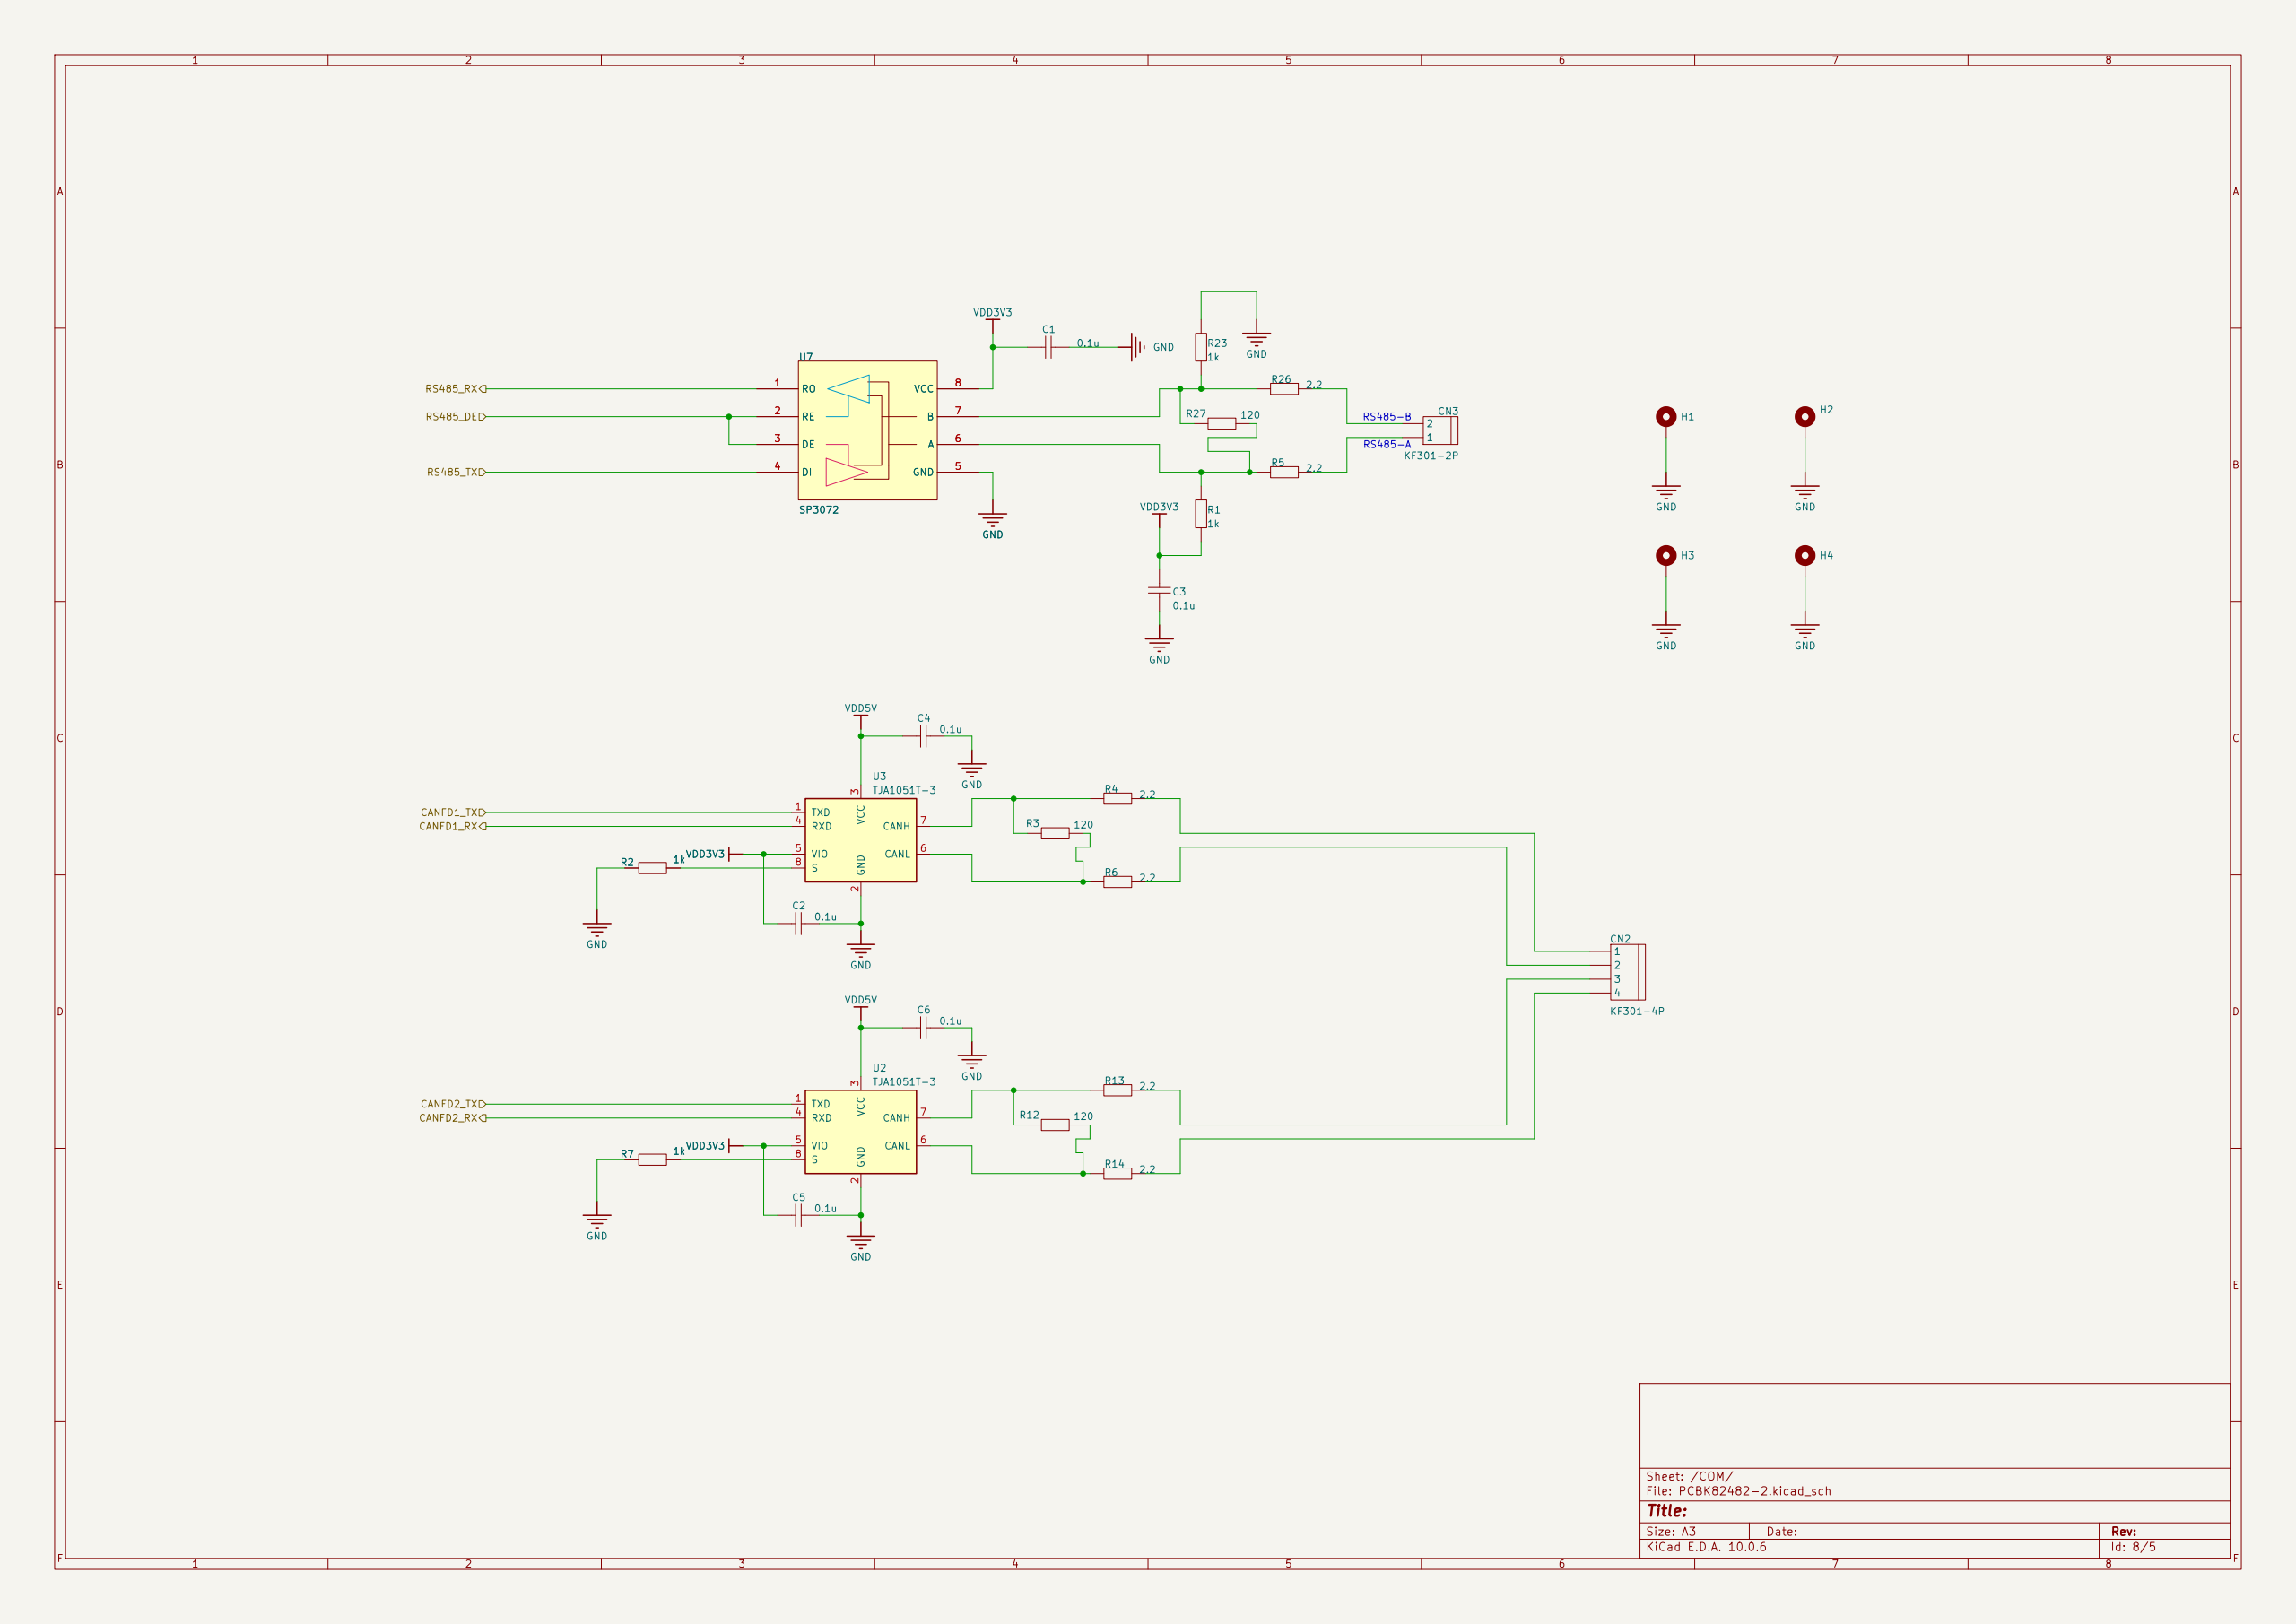Circuit board | KiCad | 154 parts | 201 nets | one sheet of the schematic
Parts on this sheet (reference | value | footprint):
C1
C2
C3
C4
C5
C6
CN3 | KF301-2P | Library:HEAD2L-0.8
H1
H2
H3
H4
R1 | 1k | Library:R0603
R12 | 120 | R0603
R13 | 2.2 | Library:R0805
R14 | 2.2 | Library:R0805
R2 | 1k | Library:R0603
R23 | 1k | Library:R0603
R26 | 2.2 | Library:R0805
R27 | 120 | R0603
R3 | 120 | R0603
R4
R5
R6
R7 | 1k | Library:R0603
U2 | TJA1051T-3 | Package_SO:SOIC-8_3.9x4.9mm_P1.27mm
U3 | TJA1051T-3 | Package_SO:SOIC-8_3.9x4.9mm_P1.27mm
U7 | SP3072 | Library:SO8_D_R-PDSO-G8
Nets of these parts (net: part-pin ...):
/Vision_Interface/BTB_RXD1: U7-1
/Vision_Interface/BTB_TXD1: U7-4
/Vision_Interface/CRX0: U3-4
/Vision_Interface/CRX1: U2-4
/Vision_Interface/CTX0: U3-1
/Vision_Interface/CTX1: U2-1
/Vision_Interface/DE1: U7-2 U7-3
GND: C1-1 C2-1 C3-2 C4-1 C5-1 C6-1 H1-1 H2-1 H3-1 H4-1 R2-1 R7-1 R23-1 U2-2 U3-2 U7-5
Net-(CN2-Pad1): R4-2
Net-(CN2-Pad2): R6-2
Net-(CN2-Pad3): R13-2
Net-(CN2-Pad4): R14-2
Net-(CN3-Pad1): CN3-1 R5-2
Net-(CN3-Pad2): CN3-2 R26-2
Net-(U2-CANH): R12-1 R13-1 U2-7
Net-(U2-CANL): R12-2 R14-1 U2-6
Net-(U2-S): R7-2 U2-8
Net-(U3-CANH): R3-1 R4-1 U3-7
Net-(U3-CANL): R3-2 R6-1 U3-6
Net-(U3-S): R2-2 U3-8
Net-(U7-A): R1-1 R5-1 R27-2 U7-6
Net-(U7-B): R23-2 R26-1 R27-1 U7-7
VDD3V3: C1-2 C2-2 C3-1 C5-2 R1-2 U2-5 U3-5 U7-8
VDD5V: C4-2 C6-2 U2-3 U3-3